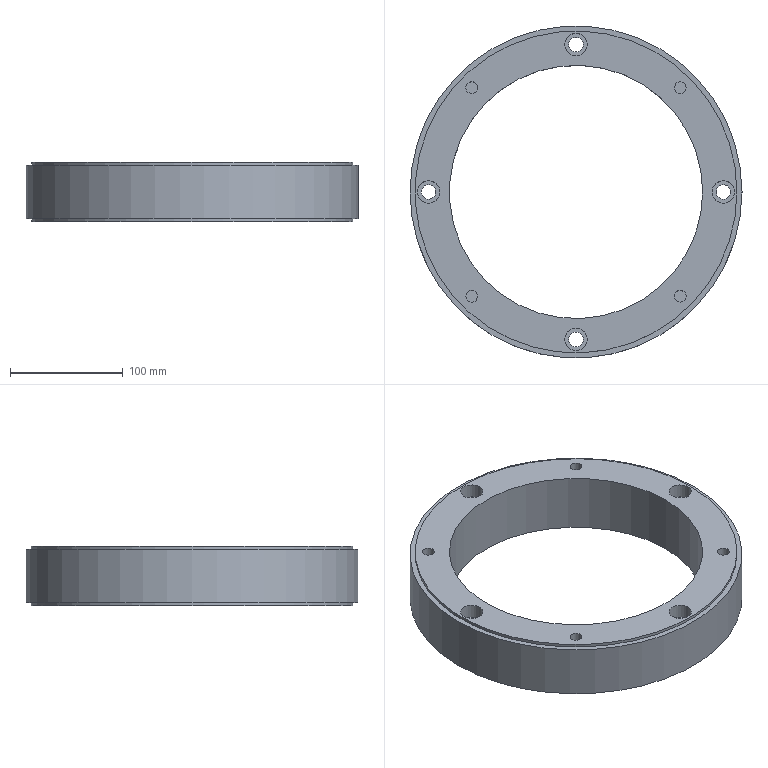NC program | NX | posted with a generic post | part box 295 x 295 x 53 mm
Whole program:
N10 G17 G21 G94 G90
(FLOOR_WALL , TOOL : D63)
N12 T01 M6
N14 G54
N16 G17 G0 G90 X-107.984 Y150.223 S6500 M3
N18 G43 Z30. H1
N20 Z3.
N22 G94 G1 Z0. F1250.
N24 X-102.759
N26 X102.756
N28 G2 X117.67 Y138.847 R181.551
N30 X125.769 Y131.555 R181.2
N32 X132.877 Y124.372 R181.91
N34 X137.181 Y119.61 R181.464
N36 G1 X-137.188
N38 G3 X-148.178 Y105.681 R181.64
N40 X-153.675 Y97.507 R180.902
N42 X-155.139 Y95.162 R181.37
N44 X-158.758 Y88.997 R181.356
N46 G1 X158.765
N48 G2 X172.394 Y58.384 R181.514
N50 G1 X-172.387
N52 G3 X-179.606 Y29.428 R181.495
N54 X-179.87 Y27.77 R180.873
N56 G1 X179.872
N58 G2 X181.102 Y18.086 R180.384
N60 X182. Y1.52 R181.116
N62 G1 Y-1.509
N64 G2 X181.984 Y-2.843 R181.116
N66 G1 X-181.981
N68 G3 X-178.903 Y-33.456 R181.304
N70 G1 X178.905
N72 G2 X177.846 Y-38.682 R180.938
N74 X174.273 Y-52.478 R181.345
N76 X170.354 Y-64.069 R180.195
N78 G1 X-170.355
N80 G3 X-155.449 Y-94.683 R183.654
N82 G1 X155.441
N84 G2 X142.768 Y-112.876 R181.305
N86 X133.99 Y-123.175 R181.019
N88 X132.011 Y-125.296 R181.556
N90 G1 X-132.012
N92 X-136.116
N94 Z3.
N96 G0 Z30.
N98 M5
(HOLE_MILLING , TOOL : D10JING)
N100 T11 M6
N102 G54
N104 G17 G0 G90 X-131. Y0. S6500 M3
N106 G43 Z30. H11
N108 Z0.5
N110 G94 G3 X-128.5 Y-2.5 R2.5 F1650.
N112 X-126. Y0. R2.5
N114 X-126. Y0. Z-0.5 I-5. J0.
N116 X-126. Y0. Z-1.5 I-5. J0.
N118 X-126. Y0. Z-2.5 I-5. J0.
N120 X-126. Y0. Z-3.5 I-5. J0.
N122 X-126. Y0. Z-4.5 I-5. J0.
N124 X-126. Y0. Z-5.5 I-5. J0.
N126 X-126. Y0. Z-6.5 I-5. J0.
N128 X-126. Y0. Z-7.5 I-5. J0.
N130 X-126. Y0. Z-8.5 I-5. J0.
N132 X-126. Y0. Z-9.5 I-5. J0.
N134 X-126. Y0. Z-10.5 I-5. J0.
N136 X-126. Y0. Z-11.5 I-5. J0.
N138 X-126. Y0. Z-12.5 I-5. J0.
N140 X-136. Y0. Z-13. I-5. J0.
N142 X-131. Y-5. R5.
N144 X-136. Y0. R-5.
N146 X-133.5 Y-2.5 R2.5
N148 X-131. Y0. R2.5
N150 G0 Z30.
N152 X0. Y-131.
N154 Z0.5
N156 G3 X2.5 Y-133.5 R2.5
N158 X5. Y-131. R2.5
N160 X5. Y-131. Z-0.5 I-5. J0.
N162 X5. Y-131. Z-1.5 I-5. J0.
N164 X5. Y-131. Z-2.5 I-5. J0.
N166 X5. Y-131. Z-3.5 I-5. J0.
N168 X5. Y-131. Z-4.5 I-5. J0.
N170 X5. Y-131. Z-5.5 I-5. J0.
N172 X5. Y-131. Z-6.5 I-5. J0.
N174 X5. Y-131. Z-7.5 I-5. J0.
N176 X5. Y-131. Z-8.5 I-5. J0.
N178 X5. Y-131. Z-9.5 I-5. J0.
N180 X5. Y-131. Z-10.5 I-5. J0.
N182 X5. Y-131. Z-11.5 I-5. J0.
N184 X5. Y-131. Z-12.5 I-5. J0.
N186 X-5. Y-131. Z-13. I-5. J0.
N188 X0. Y-136. R5.
N190 X-5. Y-131. R-5.
N192 X-2.5 Y-133.5 R2.5
N194 X0. Y-131. R2.5
N196 G0 Z30.
N198 X131. Y0.
N200 Z0.5
N202 G3 X133.5 Y-2.5 R2.5
N204 X136. Y0. R2.5
N206 X136. Y0. Z-0.5 I-5. J0.
N208 X136. Y0. Z-1.5 I-5. J0.
N210 X136. Y0. Z-2.5 I-5. J0.
N212 X136. Y0. Z-3.5 I-5. J0.
N214 X136. Y0. Z-4.5 I-5. J0.
N216 X136. Y0. Z-5.5 I-5. J0.
N218 X136. Y0. Z-6.5 I-5. J0.
N220 X136. Y0. Z-7.5 I-5. J0.
N222 X136. Y0. Z-8.5 I-5. J0.
N224 X136. Y0. Z-9.5 I-5. J0.
N226 X136. Y0. Z-10.5 I-5. J0.
N228 X136. Y0. Z-11.5 I-5. J0.
N230 X136. Y0. Z-12.5 I-5. J0.
N232 X126. Y0. Z-13. I-5. J0.
N234 X131. Y-5. R5.
N236 X126. Y0. R-5.
N238 X128.5 Y-2.5 R2.5
N240 X131. Y0. R2.5
N242 G0 Z30.
N244 X0. Y131.
N246 Z0.5
N248 G3 X2.5 Y128.5 R2.5
N250 X5. Y131. R2.5
N252 X5. Y131. Z-0.5 I-5. J0.
N254 X5. Y131. Z-1.5 I-5. J0.
N256 X5. Y131. Z-2.5 I-5. J0.
N258 X5. Y131. Z-3.5 I-5. J0.
N260 X5. Y131. Z-4.5 I-5. J0.
N262 X5. Y131. Z-5.5 I-5. J0.
N264 X5. Y131. Z-6.5 I-5. J0.
N266 X5. Y131. Z-7.5 I-5. J0.
N268 X5. Y131. Z-8.5 I-5. J0.
N270 X5. Y131. Z-9.5 I-5. J0.
N272 X5. Y131. Z-10.5 I-5. J0.
N274 X5. Y131. Z-11.5 I-5. J0.
N276 X5. Y131. Z-12.5 I-5. J0.
N278 X-5. Y131. Z-13. I-5. J0.
N280 X0. Y126. R5.
N282 X-5. Y131. R-5.
N284 X-2.5 Y128.5 R2.5
N286 X0. Y131. R2.5
N288 G0 Z30.
N290 M5
N292 M2